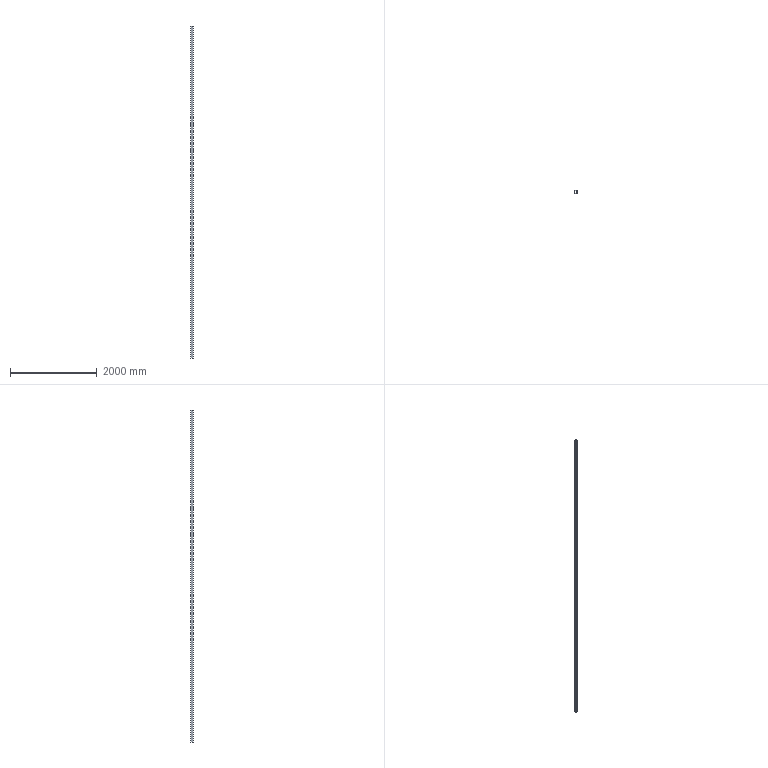Part | STEP file | 750038156 | 1 solid | 18 faces | box 60 x 60 x 7644 mm | volume 6639051 mm3 | plane 10 | cylinder 8 | commonest cylinder face diameters 4 x4 12 x4
STEP:
#1=CARTESIAN_POINT('',(-26.,24.,7644.));
#2=VERTEX_POINT('',#1);
#3=CARTESIAN_POINT('',(-26.,24.,0.));
#4=VERTEX_POINT('',#3);
#5=CARTESIAN_POINT('',(-26.,24.,7644.));
#6=DIRECTION('',(0.,0.,-1.));
#7=VECTOR('',#6,1000.);
#8=LINE('',#5,#7);
#9=EDGE_CURVE('',#2,#4,#8,.T.);
#10=ORIENTED_EDGE('',*,*,#9,.F.);
#11=CARTESIAN_POINT('',(-26.,-24.,7644.));
#12=VERTEX_POINT('',#11);
#13=CARTESIAN_POINT('',(-26.,-24.,7644.));
#14=DIRECTION('',(0.,1.,0.));
#15=VECTOR('',#14,1000.);
#16=LINE('',#13,#15);
#17=EDGE_CURVE('',#12,#2,#16,.T.);
#18=ORIENTED_EDGE('',*,*,#17,.F.);
#19=CARTESIAN_POINT('',(-26.,-24.,0.));
#20=VERTEX_POINT('',#19);
#21=CARTESIAN_POINT('',(-26.,-24.,7644.));
#22=DIRECTION('',(0.,0.,1.));
#23=VECTOR('',#22,1000.);
#24=LINE('',#21,#23);
#25=EDGE_CURVE('',#20,#12,#24,.T.);
#26=ORIENTED_EDGE('',*,*,#25,.F.);
#27=CARTESIAN_POINT('',(-26.,-24.,0.));
#28=DIRECTION('',(0.,-1.,0.));
#29=VECTOR('',#28,1000.);
#30=LINE('',#27,#29);
#31=EDGE_CURVE('',#4,#20,#30,.T.);
#32=ORIENTED_EDGE('',*,*,#31,.F.);
#33=EDGE_LOOP('',(#10,#18,#26,#32));
#34=FACE_OUTER_BOUND('',#33,.T.);
#35=CARTESIAN_POINT('',(-26.,-24.,7644.));
#36=DIRECTION('',(-1.,0.,0.));
#37=DIRECTION('',(0.,-1.,0.));
#38=AXIS2_PLACEMENT_3D('',#35,#36,#37);
#39=PLANE('',#38);
#40=ADVANCED_FACE('',(#34),#39,.F.);
#41=CARTESIAN_POINT('',(26.,24.,0.));
#42=VERTEX_POINT('',#41);
#43=CARTESIAN_POINT('',(24.,26.,0.));
#44=VERTEX_POINT('',#43);
#45=CARTESIAN_POINT('',(24.,24.,0.));
#46=DIRECTION('',(0.,0.,1.));
#47=DIRECTION('',(-1.,0.,0.));
#48=AXIS2_PLACEMENT_3D('',#45,#46,#47);
#49=CIRCLE('',#48,2.);
#50=EDGE_CURVE('',#42,#44,#49,.T.);
#51=ORIENTED_EDGE('',*,*,#50,.T.);
#52=CARTESIAN_POINT('',(-24.,26.,0.));
#53=VERTEX_POINT('',#52);
#54=CARTESIAN_POINT('',(24.,26.,0.));
#55=DIRECTION('',(-1.,0.,0.));
#56=VECTOR('',#55,1000.);
#57=LINE('',#54,#56);
#58=EDGE_CURVE('',#44,#53,#57,.T.);
#59=ORIENTED_EDGE('',*,*,#58,.T.);
#60=CARTESIAN_POINT('',(-24.,24.,0.));
#61=DIRECTION('',(0.,0.,1.));
#62=DIRECTION('',(-1.,0.,0.));
#63=AXIS2_PLACEMENT_3D('',#60,#61,#62);
#64=CIRCLE('',#63,2.);
#65=EDGE_CURVE('',#53,#4,#64,.T.);
#66=ORIENTED_EDGE('',*,*,#65,.T.);
#67=ORIENTED_EDGE('',*,*,#31,.T.);
#68=CARTESIAN_POINT('',(-24.,-26.,0.));
#69=VERTEX_POINT('',#68);
#70=CARTESIAN_POINT('',(-24.,-24.,0.));
#71=DIRECTION('',(0.,0.,1.));
#72=DIRECTION('',(-1.,0.,0.));
#73=AXIS2_PLACEMENT_3D('',#70,#71,#72);
#74=CIRCLE('',#73,2.);
#75=EDGE_CURVE('',#20,#69,#74,.T.);
#76=ORIENTED_EDGE('',*,*,#75,.T.);
#77=CARTESIAN_POINT('',(24.,-26.,0.));
#78=VERTEX_POINT('',#77);
#79=CARTESIAN_POINT('',(24.,-26.,0.));
#80=DIRECTION('',(1.,0.,0.));
#81=VECTOR('',#80,1000.);
#82=LINE('',#79,#81);
#83=EDGE_CURVE('',#69,#78,#82,.T.);
#84=ORIENTED_EDGE('',*,*,#83,.T.);
#85=CARTESIAN_POINT('',(26.,-24.,0.));
#86=VERTEX_POINT('',#85);
#87=CARTESIAN_POINT('',(24.,-24.,0.));
#88=DIRECTION('',(0.,0.,1.));
#89=DIRECTION('',(-1.,0.,0.));
#90=AXIS2_PLACEMENT_3D('',#87,#88,#89);
#91=CIRCLE('',#90,2.);
#92=EDGE_CURVE('',#78,#86,#91,.T.);
#93=ORIENTED_EDGE('',*,*,#92,.T.);
#94=CARTESIAN_POINT('',(26.,-24.,0.));
#95=DIRECTION('',(0.,1.,0.));
#96=VECTOR('',#95,1000.);
#97=LINE('',#94,#96);
#98=EDGE_CURVE('',#86,#42,#97,.T.);
#99=ORIENTED_EDGE('',*,*,#98,.T.);
#100=EDGE_LOOP('',(#51,#59,#66,#67,#76,#84,#93,#99));
#101=FACE_BOUND('',#100,.T.);
#102=CARTESIAN_POINT('',(-24.,30.,0.));
#103=VERTEX_POINT('',#102);
#104=CARTESIAN_POINT('',(24.,30.,0.));
#105=VERTEX_POINT('',#104);
#106=CARTESIAN_POINT('',(24.,30.,0.));
#107=DIRECTION('',(1.,0.,0.));
#108=VECTOR('',#107,1000.);
#109=LINE('',#106,#108);
#110=EDGE_CURVE('',#103,#105,#109,.T.);
#111=ORIENTED_EDGE('',*,*,#110,.T.);
#112=CARTESIAN_POINT('',(30.,24.,0.));
#113=VERTEX_POINT('',#112);
#114=CARTESIAN_POINT('',(24.,24.,0.));
#115=DIRECTION('',(0.,0.,-1.));
#116=DIRECTION('',(-1.,0.,0.));
#117=AXIS2_PLACEMENT_3D('',#114,#115,#116);
#118=CIRCLE('',#117,6.);
#119=EDGE_CURVE('',#105,#113,#118,.T.);
#120=ORIENTED_EDGE('',*,*,#119,.T.);
#121=CARTESIAN_POINT('',(30.,-24.,0.));
#122=VERTEX_POINT('',#121);
#123=CARTESIAN_POINT('',(30.,-24.,0.));
#124=DIRECTION('',(0.,-1.,0.));
#125=VECTOR('',#124,1000.);
#126=LINE('',#123,#125);
#127=EDGE_CURVE('',#113,#122,#126,.T.);
#128=ORIENTED_EDGE('',*,*,#127,.T.);
#129=CARTESIAN_POINT('',(24.,-30.,0.));
#130=VERTEX_POINT('',#129);
#131=CARTESIAN_POINT('',(24.,-24.,0.));
#132=DIRECTION('',(0.,0.,-1.));
#133=DIRECTION('',(-1.,0.,0.));
#134=AXIS2_PLACEMENT_3D('',#131,#132,#133);
#135=CIRCLE('',#134,6.);
#136=EDGE_CURVE('',#122,#130,#135,.T.);
#137=ORIENTED_EDGE('',*,*,#136,.T.);
#138=CARTESIAN_POINT('',(-24.,-30.,0.));
#139=VERTEX_POINT('',#138);
#140=CARTESIAN_POINT('',(24.,-30.,0.));
#141=DIRECTION('',(-1.,0.,0.));
#142=VECTOR('',#141,1000.);
#143=LINE('',#140,#142);
#144=EDGE_CURVE('',#130,#139,#143,.T.);
#145=ORIENTED_EDGE('',*,*,#144,.T.);
#146=CARTESIAN_POINT('',(-30.,-24.,0.));
#147=VERTEX_POINT('',#146);
#148=CARTESIAN_POINT('',(-24.,-24.,0.));
#149=DIRECTION('',(0.,0.,-1.));
#150=DIRECTION('',(-1.,0.,0.));
#151=AXIS2_PLACEMENT_3D('',#148,#149,#150);
#152=CIRCLE('',#151,6.);
#153=EDGE_CURVE('',#139,#147,#152,.T.);
#154=ORIENTED_EDGE('',*,*,#153,.T.);
#155=CARTESIAN_POINT('',(-30.,24.,0.));
#156=VERTEX_POINT('',#155);
#157=CARTESIAN_POINT('',(-30.,-24.,0.));
#158=DIRECTION('',(0.,1.,0.));
#159=VECTOR('',#158,1000.);
#160=LINE('',#157,#159);
#161=EDGE_CURVE('',#147,#156,#160,.T.);
#162=ORIENTED_EDGE('',*,*,#161,.T.);
#163=CARTESIAN_POINT('',(-24.,24.,0.));
#164=DIRECTION('',(0.,0.,-1.));
#165=DIRECTION('',(-1.,0.,0.));
#166=AXIS2_PLACEMENT_3D('',#163,#164,#165);
#167=CIRCLE('',#166,6.);
#168=EDGE_CURVE('',#156,#103,#167,.T.);
#169=ORIENTED_EDGE('',*,*,#168,.T.);
#170=EDGE_LOOP('',(#111,#120,#128,#137,#145,#154,#162,#169));
#171=FACE_OUTER_BOUND('',#170,.T.);
#172=CARTESIAN_POINT('',(24.,-24.,0.));
#173=DIRECTION('',(0.,0.,-1.));
#174=DIRECTION('',(-1.,0.,0.));
#175=AXIS2_PLACEMENT_3D('',#172,#173,#174);
#176=PLANE('',#175);
#177=ADVANCED_FACE('',(#101,#171),#176,.T.);
#178=CARTESIAN_POINT('',(-24.,26.,7644.));
#179=VERTEX_POINT('',#178);
#180=CARTESIAN_POINT('',(-24.,26.,7644.));
#181=DIRECTION('',(0.,0.,-1.));
#182=VECTOR('',#181,1000.);
#183=LINE('',#180,#182);
#184=EDGE_CURVE('',#179,#53,#183,.T.);
#185=ORIENTED_EDGE('',*,*,#184,.F.);
#186=CARTESIAN_POINT('',(-24.,24.,7644.));
#187=DIRECTION('',(0.,0.,-1.));
#188=DIRECTION('',(-1.,0.,0.));
#189=AXIS2_PLACEMENT_3D('',#186,#187,#188);
#190=CIRCLE('',#189,2.);
#191=EDGE_CURVE('',#2,#179,#190,.T.);
#192=ORIENTED_EDGE('',*,*,#191,.F.);
#193=ORIENTED_EDGE('',*,*,#9,.T.);
#194=ORIENTED_EDGE('',*,*,#65,.F.);
#195=EDGE_LOOP('',(#185,#192,#193,#194));
#196=FACE_OUTER_BOUND('',#195,.T.);
#197=CARTESIAN_POINT('',(-24.,24.,7644.));
#198=DIRECTION('',(0.,0.,-1.));
#199=DIRECTION('',(-1.,0.,0.));
#200=AXIS2_PLACEMENT_3D('',#197,#198,#199);
#201=CYLINDRICAL_SURFACE('',#200,2.);
#202=ADVANCED_FACE('',(#196),#201,.F.);
#203=CARTESIAN_POINT('',(24.,26.,7644.));
#204=VERTEX_POINT('',#203);
#205=CARTESIAN_POINT('',(24.,26.,7644.));
#206=DIRECTION('',(-1.,0.,0.));
#207=VECTOR('',#206,1000.);
#208=LINE('',#205,#207);
#209=EDGE_CURVE('',#204,#179,#208,.T.);
#210=ORIENTED_EDGE('',*,*,#209,.F.);
#211=CARTESIAN_POINT('',(26.,24.,7644.));
#212=VERTEX_POINT('',#211);
#213=CARTESIAN_POINT('',(24.,24.,7644.));
#214=DIRECTION('',(0.,0.,1.));
#215=DIRECTION('',(-1.,0.,0.));
#216=AXIS2_PLACEMENT_3D('',#213,#214,#215);
#217=CIRCLE('',#216,2.);
#218=EDGE_CURVE('',#212,#204,#217,.T.);
#219=ORIENTED_EDGE('',*,*,#218,.F.);
#220=CARTESIAN_POINT('',(26.,-24.,7644.));
#221=VERTEX_POINT('',#220);
#222=CARTESIAN_POINT('',(26.,-24.,7644.));
#223=DIRECTION('',(0.,1.,0.));
#224=VECTOR('',#223,1000.);
#225=LINE('',#222,#224);
#226=EDGE_CURVE('',#221,#212,#225,.T.);
#227=ORIENTED_EDGE('',*,*,#226,.F.);
#228=CARTESIAN_POINT('',(24.,-26.,7644.));
#229=VERTEX_POINT('',#228);
#230=CARTESIAN_POINT('',(24.,-24.,7644.));
#231=DIRECTION('',(0.,0.,1.));
#232=DIRECTION('',(-1.,0.,0.));
#233=AXIS2_PLACEMENT_3D('',#230,#231,#232);
#234=CIRCLE('',#233,2.);
#235=EDGE_CURVE('',#229,#221,#234,.T.);
#236=ORIENTED_EDGE('',*,*,#235,.F.);
#237=CARTESIAN_POINT('',(-24.,-26.,7644.));
#238=VERTEX_POINT('',#237);
#239=CARTESIAN_POINT('',(24.,-26.,7644.));
#240=DIRECTION('',(1.,0.,0.));
#241=VECTOR('',#240,1000.);
#242=LINE('',#239,#241);
#243=EDGE_CURVE('',#238,#229,#242,.T.);
#244=ORIENTED_EDGE('',*,*,#243,.F.);
#245=CARTESIAN_POINT('',(-24.,-24.,7644.));
#246=DIRECTION('',(0.,0.,1.));
#247=DIRECTION('',(-1.,0.,0.));
#248=AXIS2_PLACEMENT_3D('',#245,#246,#247);
#249=CIRCLE('',#248,2.);
#250=EDGE_CURVE('',#12,#238,#249,.T.);
#251=ORIENTED_EDGE('',*,*,#250,.F.);
#252=ORIENTED_EDGE('',*,*,#17,.T.);
#253=ORIENTED_EDGE('',*,*,#191,.T.);
#254=EDGE_LOOP('',(#210,#219,#227,#236,#244,#251,#252,#253));
#255=FACE_BOUND('',#254,.T.);
#256=CARTESIAN_POINT('',(24.,30.,7644.));
#257=VERTEX_POINT('',#256);
#258=CARTESIAN_POINT('',(30.,24.,7644.));
#259=VERTEX_POINT('',#258);
#260=CARTESIAN_POINT('',(24.,24.,7644.));
#261=DIRECTION('',(0.,0.,-1.));
#262=DIRECTION('',(-1.,0.,0.));
#263=AXIS2_PLACEMENT_3D('',#260,#261,#262);
#264=CIRCLE('',#263,6.);
#265=EDGE_CURVE('',#257,#259,#264,.T.);
#266=ORIENTED_EDGE('',*,*,#265,.F.);
#267=CARTESIAN_POINT('',(-24.,30.,7644.));
#268=VERTEX_POINT('',#267);
#269=CARTESIAN_POINT('',(24.,30.,7644.));
#270=DIRECTION('',(1.,0.,0.));
#271=VECTOR('',#270,1000.);
#272=LINE('',#269,#271);
#273=EDGE_CURVE('',#268,#257,#272,.T.);
#274=ORIENTED_EDGE('',*,*,#273,.F.);
#275=CARTESIAN_POINT('',(-30.,24.,7644.));
#276=VERTEX_POINT('',#275);
#277=CARTESIAN_POINT('',(-24.,24.,7644.));
#278=DIRECTION('',(0.,0.,-1.));
#279=DIRECTION('',(-1.,0.,0.));
#280=AXIS2_PLACEMENT_3D('',#277,#278,#279);
#281=CIRCLE('',#280,6.);
#282=EDGE_CURVE('',#276,#268,#281,.T.);
#283=ORIENTED_EDGE('',*,*,#282,.F.);
#284=CARTESIAN_POINT('',(-30.,-24.,7644.));
#285=VERTEX_POINT('',#284);
#286=CARTESIAN_POINT('',(-30.,-24.,7644.));
#287=DIRECTION('',(0.,1.,0.));
#288=VECTOR('',#287,1000.);
#289=LINE('',#286,#288);
#290=EDGE_CURVE('',#285,#276,#289,.T.);
#291=ORIENTED_EDGE('',*,*,#290,.F.);
#292=CARTESIAN_POINT('',(-24.,-30.,7644.));
#293=VERTEX_POINT('',#292);
#294=CARTESIAN_POINT('',(-24.,-24.,7644.));
#295=DIRECTION('',(0.,0.,-1.));
#296=DIRECTION('',(-1.,0.,0.));
#297=AXIS2_PLACEMENT_3D('',#294,#295,#296);
#298=CIRCLE('',#297,6.);
#299=EDGE_CURVE('',#293,#285,#298,.T.);
#300=ORIENTED_EDGE('',*,*,#299,.F.);
#301=CARTESIAN_POINT('',(24.,-30.,7644.));
#302=VERTEX_POINT('',#301);
#303=CARTESIAN_POINT('',(24.,-30.,7644.));
#304=DIRECTION('',(-1.,0.,0.));
#305=VECTOR('',#304,1000.);
#306=LINE('',#303,#305);
#307=EDGE_CURVE('',#302,#293,#306,.T.);
#308=ORIENTED_EDGE('',*,*,#307,.F.);
#309=CARTESIAN_POINT('',(30.,-24.,7644.));
#310=VERTEX_POINT('',#309);
#311=CARTESIAN_POINT('',(24.,-24.,7644.));
#312=DIRECTION('',(0.,0.,-1.));
#313=DIRECTION('',(-1.,0.,0.));
#314=AXIS2_PLACEMENT_3D('',#311,#312,#313);
#315=CIRCLE('',#314,6.);
#316=EDGE_CURVE('',#310,#302,#315,.T.);
#317=ORIENTED_EDGE('',*,*,#316,.F.);
#318=CARTESIAN_POINT('',(30.,-24.,7644.));
#319=DIRECTION('',(0.,-1.,0.));
#320=VECTOR('',#319,1000.);
#321=LINE('',#318,#320);
#322=EDGE_CURVE('',#259,#310,#321,.T.);
#323=ORIENTED_EDGE('',*,*,#322,.F.);
#324=EDGE_LOOP('',(#266,#274,#283,#291,#300,#308,#317,#323));
#325=FACE_OUTER_BOUND('',#324,.T.);
#326=CARTESIAN_POINT('',(24.,-24.,7644.));
#327=DIRECTION('',(0.,0.,-1.));
#328=DIRECTION('',(-1.,0.,0.));
#329=AXIS2_PLACEMENT_3D('',#326,#327,#328);
#330=PLANE('',#329);
#331=ADVANCED_FACE('',(#255,#325),#330,.F.);
#332=ORIENTED_EDGE('',*,*,#25,.T.);
#333=ORIENTED_EDGE('',*,*,#250,.T.);
#334=CARTESIAN_POINT('',(-24.,-26.,7644.));
#335=DIRECTION('',(0.,0.,1.));
#336=VECTOR('',#335,1000.);
#337=LINE('',#334,#336);
#338=EDGE_CURVE('',#69,#238,#337,.T.);
#339=ORIENTED_EDGE('',*,*,#338,.F.);
#340=ORIENTED_EDGE('',*,*,#75,.F.);
#341=EDGE_LOOP('',(#332,#333,#339,#340));
#342=FACE_OUTER_BOUND('',#341,.T.);
#343=CARTESIAN_POINT('',(-24.,-24.,7644.));
#344=DIRECTION('',(0.,0.,-1.));
#345=DIRECTION('',(-1.,0.,0.));
#346=AXIS2_PLACEMENT_3D('',#343,#344,#345);
#347=CYLINDRICAL_SURFACE('',#346,2.);
#348=ADVANCED_FACE('',(#342),#347,.F.);
#349=CARTESIAN_POINT('',(24.,26.,7644.));
#350=DIRECTION('',(0.,0.,-1.));
#351=VECTOR('',#350,1000.);
#352=LINE('',#349,#351);
#353=EDGE_CURVE('',#204,#44,#352,.T.);
#354=ORIENTED_EDGE('',*,*,#353,.F.);
#355=ORIENTED_EDGE('',*,*,#209,.T.);
#356=ORIENTED_EDGE('',*,*,#184,.T.);
#357=ORIENTED_EDGE('',*,*,#58,.F.);
#358=EDGE_LOOP('',(#354,#355,#356,#357));
#359=FACE_OUTER_BOUND('',#358,.T.);
#360=CARTESIAN_POINT('',(-24.,26.,7644.));
#361=DIRECTION('',(0.,1.,0.));
#362=DIRECTION('',(0.,0.,1.));
#363=AXIS2_PLACEMENT_3D('',#360,#361,#362);
#364=PLANE('',#363);
#365=ADVANCED_FACE('',(#359),#364,.F.);
#366=CARTESIAN_POINT('',(26.,24.,7644.));
#367=DIRECTION('',(0.,0.,-1.));
#368=VECTOR('',#367,1000.);
#369=LINE('',#366,#368);
#370=EDGE_CURVE('',#212,#42,#369,.T.);
#371=ORIENTED_EDGE('',*,*,#370,.F.);
#372=ORIENTED_EDGE('',*,*,#218,.T.);
#373=ORIENTED_EDGE('',*,*,#353,.T.);
#374=ORIENTED_EDGE('',*,*,#50,.F.);
#375=EDGE_LOOP('',(#371,#372,#373,#374));
#376=FACE_OUTER_BOUND('',#375,.T.);
#377=CARTESIAN_POINT('',(24.,24.,7644.));
#378=DIRECTION('',(0.,0.,-1.));
#379=DIRECTION('',(-1.,0.,0.));
#380=AXIS2_PLACEMENT_3D('',#377,#378,#379);
#381=CYLINDRICAL_SURFACE('',#380,2.);
#382=ADVANCED_FACE('',(#376),#381,.F.);
#383=CARTESIAN_POINT('',(26.,-24.,7644.));
#384=DIRECTION('',(0.,0.,-1.));
#385=VECTOR('',#384,1000.);
#386=LINE('',#383,#385);
#387=EDGE_CURVE('',#221,#86,#386,.T.);
#388=ORIENTED_EDGE('',*,*,#387,.F.);
#389=ORIENTED_EDGE('',*,*,#226,.T.);
#390=ORIENTED_EDGE('',*,*,#370,.T.);
#391=ORIENTED_EDGE('',*,*,#98,.F.);
#392=EDGE_LOOP('',(#388,#389,#390,#391));
#393=FACE_OUTER_BOUND('',#392,.T.);
#394=CARTESIAN_POINT('',(26.,24.,7644.));
#395=DIRECTION('',(1.,0.,0.));
#396=DIRECTION('',(0.,0.,-1.));
#397=AXIS2_PLACEMENT_3D('',#394,#395,#396);
#398=PLANE('',#397);
#399=ADVANCED_FACE('',(#393),#398,.F.);
#400=CARTESIAN_POINT('',(24.,-26.,7644.));
#401=DIRECTION('',(0.,0.,-1.));
#402=VECTOR('',#401,1000.);
#403=LINE('',#400,#402);
#404=EDGE_CURVE('',#229,#78,#403,.T.);
#405=ORIENTED_EDGE('',*,*,#404,.F.);
#406=ORIENTED_EDGE('',*,*,#235,.T.);
#407=ORIENTED_EDGE('',*,*,#387,.T.);
#408=ORIENTED_EDGE('',*,*,#92,.F.);
#409=EDGE_LOOP('',(#405,#406,#407,#408));
#410=FACE_OUTER_BOUND('',#409,.T.);
#411=CARTESIAN_POINT('',(24.,-24.,7644.));
#412=DIRECTION('',(0.,0.,-1.));
#413=DIRECTION('',(-1.,0.,0.));
#414=AXIS2_PLACEMENT_3D('',#411,#412,#413);
#415=CYLINDRICAL_SURFACE('',#414,2.);
#416=ADVANCED_FACE('',(#410),#415,.F.);
#417=ORIENTED_EDGE('',*,*,#338,.T.);
#418=ORIENTED_EDGE('',*,*,#243,.T.);
#419=ORIENTED_EDGE('',*,*,#404,.T.);
#420=ORIENTED_EDGE('',*,*,#83,.F.);
#421=EDGE_LOOP('',(#417,#418,#419,#420));
#422=FACE_OUTER_BOUND('',#421,.T.);
#423=CARTESIAN_POINT('',(24.,-26.,7644.));
#424=DIRECTION('',(0.,-1.,0.));
#425=DIRECTION('',(0.,0.,-1.));
#426=AXIS2_PLACEMENT_3D('',#423,#424,#425);
#427=PLANE('',#426);
#428=ADVANCED_FACE('',(#422),#427,.F.);
#429=ORIENTED_EDGE('',*,*,#265,.T.);
#430=CARTESIAN_POINT('',(30.,24.,7644.));
#431=DIRECTION('',(0.,0.,-1.));
#432=VECTOR('',#431,1000.);
#433=LINE('',#430,#432);
#434=EDGE_CURVE('',#259,#113,#433,.T.);
#435=ORIENTED_EDGE('',*,*,#434,.T.);
#436=ORIENTED_EDGE('',*,*,#119,.F.);
#437=CARTESIAN_POINT('',(24.,30.,7644.));
#438=DIRECTION('',(0.,0.,1.));
#439=VECTOR('',#438,1000.);
#440=LINE('',#437,#439);
#441=EDGE_CURVE('',#105,#257,#440,.T.);
#442=ORIENTED_EDGE('',*,*,#441,.T.);
#443=EDGE_LOOP('',(#429,#435,#436,#442));
#444=FACE_OUTER_BOUND('',#443,.T.);
#445=CARTESIAN_POINT('',(24.,24.,7644.));
#446=DIRECTION('',(0.,0.,-1.));
#447=DIRECTION('',(-1.,0.,0.));
#448=AXIS2_PLACEMENT_3D('',#445,#446,#447);
#449=CYLINDRICAL_SURFACE('',#448,6.);
#450=ADVANCED_FACE('',(#444),#449,.T.);
#451=ORIENTED_EDGE('',*,*,#273,.T.);
#452=ORIENTED_EDGE('',*,*,#441,.F.);
#453=ORIENTED_EDGE('',*,*,#110,.F.);
#454=CARTESIAN_POINT('',(-24.,30.,7644.));
#455=DIRECTION('',(0.,0.,1.));
#456=VECTOR('',#455,1000.);
#457=LINE('',#454,#456);
#458=EDGE_CURVE('',#103,#268,#457,.T.);
#459=ORIENTED_EDGE('',*,*,#458,.T.);
#460=EDGE_LOOP('',(#451,#452,#453,#459));
#461=FACE_OUTER_BOUND('',#460,.T.);
#462=CARTESIAN_POINT('',(-24.,30.,7644.));
#463=DIRECTION('',(0.,1.,0.));
#464=DIRECTION('',(-1.,0.,0.));
#465=AXIS2_PLACEMENT_3D('',#462,#463,#464);
#466=PLANE('',#465);
#467=ADVANCED_FACE('',(#461),#466,.T.);
#468=ORIENTED_EDGE('',*,*,#282,.T.);
#469=ORIENTED_EDGE('',*,*,#458,.F.);
#470=ORIENTED_EDGE('',*,*,#168,.F.);
#471=CARTESIAN_POINT('',(-30.,24.,7644.));
#472=DIRECTION('',(0.,0.,1.));
#473=VECTOR('',#472,1000.);
#474=LINE('',#471,#473);
#475=EDGE_CURVE('',#156,#276,#474,.T.);
#476=ORIENTED_EDGE('',*,*,#475,.T.);
#477=EDGE_LOOP('',(#468,#469,#470,#476));
#478=FACE_OUTER_BOUND('',#477,.T.);
#479=CARTESIAN_POINT('',(-24.,24.,7644.));
#480=DIRECTION('',(0.,0.,-1.));
#481=DIRECTION('',(-1.,0.,0.));
#482=AXIS2_PLACEMENT_3D('',#479,#480,#481);
#483=CYLINDRICAL_SURFACE('',#482,6.);
#484=ADVANCED_FACE('',(#478),#483,.T.);
#485=ORIENTED_EDGE('',*,*,#290,.T.);
#486=ORIENTED_EDGE('',*,*,#475,.F.);
#487=ORIENTED_EDGE('',*,*,#161,.F.);
#488=CARTESIAN_POINT('',(-30.,-24.,7644.));
#489=DIRECTION('',(0.,0.,1.));
#490=VECTOR('',#489,1000.);
#491=LINE('',#488,#490);
#492=EDGE_CURVE('',#147,#285,#491,.T.);
#493=ORIENTED_EDGE('',*,*,#492,.T.);
#494=EDGE_LOOP('',(#485,#486,#487,#493));
#495=FACE_OUTER_BOUND('',#494,.T.);
#496=CARTESIAN_POINT('',(-30.,-24.,7644.));
#497=DIRECTION('',(-1.,0.,0.));
#498=DIRECTION('',(0.,-1.,0.));
#499=AXIS2_PLACEMENT_3D('',#496,#497,#498);
#500=PLANE('',#499);
#501=ADVANCED_FACE('',(#495),#500,.T.);
#502=ORIENTED_EDGE('',*,*,#299,.T.);
#503=ORIENTED_EDGE('',*,*,#492,.F.);
#504=ORIENTED_EDGE('',*,*,#153,.F.);
#505=CARTESIAN_POINT('',(-24.,-30.,7644.));
#506=DIRECTION('',(0.,0.,1.));
#507=VECTOR('',#506,1000.);
#508=LINE('',#505,#507);
#509=EDGE_CURVE('',#139,#293,#508,.T.);
#510=ORIENTED_EDGE('',*,*,#509,.T.);
#511=EDGE_LOOP('',(#502,#503,#504,#510));
#512=FACE_OUTER_BOUND('',#511,.T.);
#513=CARTESIAN_POINT('',(-24.,-24.,7644.));
#514=DIRECTION('',(0.,0.,-1.));
#515=DIRECTION('',(-1.,0.,0.));
#516=AXIS2_PLACEMENT_3D('',#513,#514,#515);
#517=CYLINDRICAL_SURFACE('',#516,6.);
#518=ADVANCED_FACE('',(#512),#517,.T.);
#519=ORIENTED_EDGE('',*,*,#307,.T.);
#520=ORIENTED_EDGE('',*,*,#509,.F.);
#521=ORIENTED_EDGE('',*,*,#144,.F.);
#522=CARTESIAN_POINT('',(24.,-30.,7644.));
#523=DIRECTION('',(0.,0.,1.));
#524=VECTOR('',#523,1000.);
#525=LINE('',#522,#524);
#526=EDGE_CURVE('',#130,#302,#525,.T.);
#527=ORIENTED_EDGE('',*,*,#526,.T.);
#528=EDGE_LOOP('',(#519,#520,#521,#527));
#529=FACE_OUTER_BOUND('',#528,.T.);
#530=CARTESIAN_POINT('',(24.,-30.,7644.));
#531=DIRECTION('',(0.,-1.,0.));
#532=DIRECTION('',(1.,0.,0.));
#533=AXIS2_PLACEMENT_3D('',#530,#531,#532);
#534=PLANE('',#533);
#535=ADVANCED_FACE('',(#529),#534,.T.);
#536=ORIENTED_EDGE('',*,*,#316,.T.);
#537=ORIENTED_EDGE('',*,*,#526,.F.);
#538=ORIENTED_EDGE('',*,*,#136,.F.);
#539=CARTESIAN_POINT('',(30.,-24.,7644.));
#540=DIRECTION('',(0.,0.,1.));
#541=VECTOR('',#540,1000.);
#542=LINE('',#539,#541);
#543=EDGE_CURVE('',#122,#310,#542,.T.);
#544=ORIENTED_EDGE('',*,*,#543,.T.);
#545=EDGE_LOOP('',(#536,#537,#538,#544));
#546=FACE_OUTER_BOUND('',#545,.T.);
#547=CARTESIAN_POINT('',(24.,-24.,7644.));
#548=DIRECTION('',(0.,0.,-1.));
#549=DIRECTION('',(-1.,0.,0.));
#550=AXIS2_PLACEMENT_3D('',#547,#548,#549);
#551=CYLINDRICAL_SURFACE('',#550,6.);
#552=ADVANCED_FACE('',(#546),#551,.T.);
#553=ORIENTED_EDGE('',*,*,#322,.T.);
#554=ORIENTED_EDGE('',*,*,#543,.F.);
#555=ORIENTED_EDGE('',*,*,#127,.F.);
#556=ORIENTED_EDGE('',*,*,#434,.F.);
#557=EDGE_LOOP('',(#553,#554,#555,#556));
#558=FACE_OUTER_BOUND('',#557,.T.);
#559=CARTESIAN_POINT('',(30.,24.,7644.));
#560=DIRECTION('',(1.,0.,0.));
#561=DIRECTION('',(0.,0.,-1.));
#562=AXIS2_PLACEMENT_3D('',#559,#560,#561);
#563=PLANE('',#562);
#564=ADVANCED_FACE('',(#558),#563,.T.);
#565=CLOSED_SHELL('',(#40,#177,#202,#331,#348,#365,#382,#399,#416,#428,#450,#467,#484,#501,#518,#535,#552,#564));
#566=MANIFOLD_SOLID_BREP('',#565);
#567=CARTESIAN_POINT('',(0.,0.,0.));
#568=DIRECTION('',(0.,0.,1.));
#569=DIRECTION('',(1.,0.,0.));
#570=AXIS2_PLACEMENT_3D('',#567,#568,#569);
#571=(LENGTH_UNIT()NAMED_UNIT(*)SI_UNIT(.MILLI.,.METRE.));
#572=UNCERTAINTY_MEASURE_WITH_UNIT(LENGTH_MEASURE(0.00001),#571,'','');
#573=(NAMED_UNIT(*)PLANE_ANGLE_UNIT()SI_UNIT($,.RADIAN.));
#574=(NAMED_UNIT(*)SI_UNIT($,.STERADIAN.)SOLID_ANGLE_UNIT());
#575=(GEOMETRIC_REPRESENTATION_CONTEXT(3)GLOBAL_UNCERTAINTY_ASSIGNED_CONTEXT((#572))GLOBAL_UNIT_ASSIGNED_CONTEXT((#571,#573,#574))REPRESENTATION_CONTEXT('',''));
#576=ADVANCED_BREP_SHAPE_REPRESENTATION('',(#566,#570),#575);